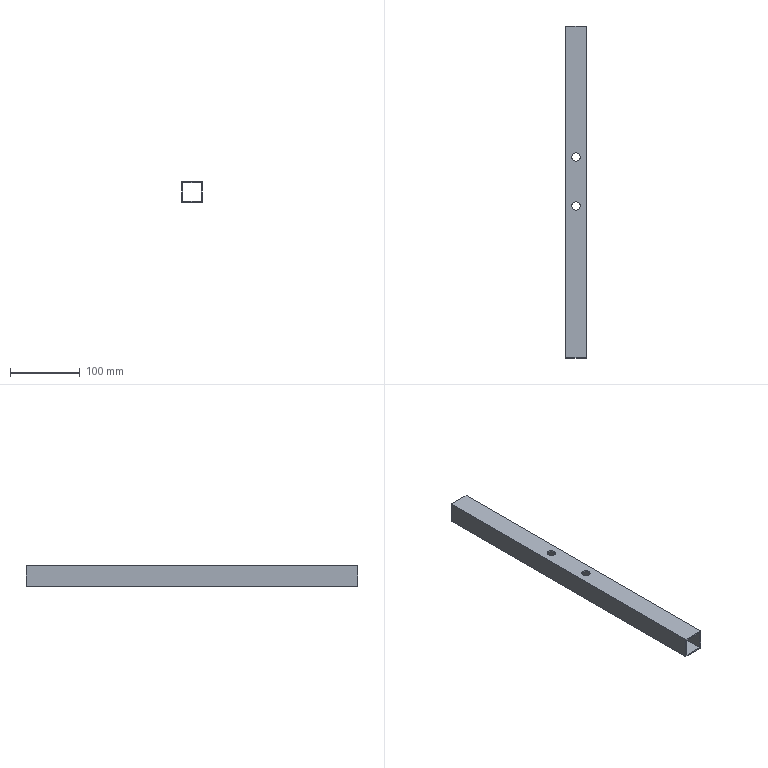Part | NX | features solid 2 | 1 solid | 14 faces | box 30 x 475 x 30 mm | volume 105495 mm3 | plane 10 | cylinder 4 | commonest cylinder face diameters 12 x4
STEP:
#1=CARTESIAN_POINT('',(240.,300.,-15.));
#2=VERTEX_POINT('',#1);
#3=CARTESIAN_POINT('',(270.,300.,-15.));
#4=VERTEX_POINT('',#3);
#5=CARTESIAN_POINT('',(270.,300.,-15.));
#6=DIRECTION('',(-1.,0.,0.));
#7=VECTOR('',#6,1000.);
#8=LINE('',#5,#7);
#9=EDGE_CURVE('',#2,#4,#8,.F.);
#10=ORIENTED_EDGE('',*,*,#9,.F.);
#11=CARTESIAN_POINT('',(240.,-175.,-15.));
#12=VERTEX_POINT('',#11);
#13=CARTESIAN_POINT('',(240.,40.,-15.));
#14=DIRECTION('',(0.,1.,0.));
#15=VECTOR('',#14,1000.);
#16=LINE('',#13,#15);
#17=EDGE_CURVE('',#12,#2,#16,.T.);
#18=ORIENTED_EDGE('',*,*,#17,.F.);
#19=CARTESIAN_POINT('',(270.,-175.,-15.));
#20=VERTEX_POINT('',#19);
#21=CARTESIAN_POINT('',(25.,-175.,-15.));
#22=DIRECTION('',(1.,0.,0.));
#23=VECTOR('',#22,1000.);
#24=LINE('',#21,#23);
#25=EDGE_CURVE('',#20,#12,#24,.F.);
#26=ORIENTED_EDGE('',*,*,#25,.F.);
#27=CARTESIAN_POINT('',(270.,40.,-15.));
#28=DIRECTION('',(0.,1.,0.));
#29=VECTOR('',#28,1000.);
#30=LINE('',#27,#29);
#31=EDGE_CURVE('',#20,#4,#30,.T.);
#32=ORIENTED_EDGE('',*,*,#31,.T.);
#33=EDGE_LOOP('',(#10,#18,#26,#32));
#34=FACE_BOUND('',#33,.T.);
#35=CARTESIAN_POINT('',(249.,112.5,-15.));
#36=VERTEX_POINT('',#35);
#37=CARTESIAN_POINT('',(255.,112.5,-15.));
#38=DIRECTION('',(0.,0.,-1.));
#39=DIRECTION('',(-1.,0.,0.));
#40=AXIS2_PLACEMENT_3D('',#37,#38,#39);
#41=CIRCLE('',#40,6.);
#42=EDGE_CURVE('',#36,#36,#41,.T.);
#43=ORIENTED_EDGE('',*,*,#42,.T.);
#44=EDGE_LOOP('',(#43));
#45=FACE_BOUND('',#44,.T.);
#46=CARTESIAN_POINT('',(249.,42.5,-15.));
#47=VERTEX_POINT('',#46);
#48=CARTESIAN_POINT('',(255.,42.5,-15.));
#49=DIRECTION('',(0.,0.,-1.));
#50=DIRECTION('',(-1.,0.,0.));
#51=AXIS2_PLACEMENT_3D('',#48,#49,#50);
#52=CIRCLE('',#51,6.);
#53=EDGE_CURVE('',#47,#47,#52,.F.);
#54=ORIENTED_EDGE('',*,*,#53,.F.);
#55=EDGE_LOOP('',(#54));
#56=FACE_BOUND('',#55,.T.);
#57=CARTESIAN_POINT('',(270.,40.,-15.));
#58=DIRECTION('',(0.,0.,-1.));
#59=DIRECTION('',(0.,1.,0.));
#60=AXIS2_PLACEMENT_3D('',#57,#58,#59);
#61=PLANE('',#60);
#62=ADVANCED_FACE('',(#34,#45,#56),#61,.F.);
#63=CARTESIAN_POINT('',(240.,-175.,-45.));
#64=VERTEX_POINT('',#63);
#65=CARTESIAN_POINT('',(240.,300.,-45.));
#66=VERTEX_POINT('',#65);
#67=CARTESIAN_POINT('',(240.,40.,-45.));
#68=DIRECTION('',(0.,1.,0.));
#69=VECTOR('',#68,1000.);
#70=LINE('',#67,#69);
#71=EDGE_CURVE('',#64,#66,#70,.T.);
#72=ORIENTED_EDGE('',*,*,#71,.T.);
#73=CARTESIAN_POINT('',(270.,300.,-45.));
#74=VERTEX_POINT('',#73);
#75=CARTESIAN_POINT('',(270.,300.,-45.));
#76=DIRECTION('',(-1.,0.,0.));
#77=VECTOR('',#76,1000.);
#78=LINE('',#75,#77);
#79=EDGE_CURVE('',#74,#66,#78,.T.);
#80=ORIENTED_EDGE('',*,*,#79,.F.);
#81=CARTESIAN_POINT('',(270.,-175.,-45.));
#82=VERTEX_POINT('',#81);
#83=CARTESIAN_POINT('',(270.,40.,-45.));
#84=DIRECTION('',(0.,1.,0.));
#85=VECTOR('',#84,1000.);
#86=LINE('',#83,#85);
#87=EDGE_CURVE('',#82,#74,#86,.T.);
#88=ORIENTED_EDGE('',*,*,#87,.F.);
#89=CARTESIAN_POINT('',(270.,-175.,-45.));
#90=DIRECTION('',(-1.,0.,0.));
#91=VECTOR('',#90,1000.);
#92=LINE('',#89,#91);
#93=EDGE_CURVE('',#82,#64,#92,.T.);
#94=ORIENTED_EDGE('',*,*,#93,.T.);
#95=EDGE_LOOP('',(#72,#80,#88,#94));
#96=FACE_BOUND('',#95,.T.);
#97=CARTESIAN_POINT('',(261.,112.5,-45.));
#98=VERTEX_POINT('',#97);
#99=CARTESIAN_POINT('',(255.,112.5,-45.));
#100=DIRECTION('',(0.,0.,-1.));
#101=DIRECTION('',(1.,0.,0.));
#102=AXIS2_PLACEMENT_3D('',#99,#100,#101);
#103=CIRCLE('',#102,6.);
#104=EDGE_CURVE('',#98,#98,#103,.T.);
#105=ORIENTED_EDGE('',*,*,#104,.F.);
#106=EDGE_LOOP('',(#105));
#107=FACE_BOUND('',#106,.T.);
#108=CARTESIAN_POINT('',(261.,42.5,-45.));
#109=VERTEX_POINT('',#108);
#110=CARTESIAN_POINT('',(255.,42.5,-45.));
#111=DIRECTION('',(0.,0.,1.));
#112=DIRECTION('',(1.,0.,0.));
#113=AXIS2_PLACEMENT_3D('',#110,#111,#112);
#114=CIRCLE('',#113,6.);
#115=EDGE_CURVE('',#109,#109,#114,.T.);
#116=ORIENTED_EDGE('',*,*,#115,.T.);
#117=EDGE_LOOP('',(#116));
#118=FACE_BOUND('',#117,.T.);
#119=CARTESIAN_POINT('',(270.,40.,-45.));
#120=DIRECTION('',(0.,0.,-1.));
#121=DIRECTION('',(0.,1.,0.));
#122=AXIS2_PLACEMENT_3D('',#119,#120,#121);
#123=PLANE('',#122);
#124=ADVANCED_FACE('',(#96,#107,#118),#123,.T.);
#125=CARTESIAN_POINT('',(242.,-175.,-17.));
#126=VERTEX_POINT('',#125);
#127=CARTESIAN_POINT('',(242.,300.,-17.));
#128=VERTEX_POINT('',#127);
#129=CARTESIAN_POINT('',(242.,40.,-17.));
#130=DIRECTION('',(0.,1.,0.));
#131=VECTOR('',#130,1000.);
#132=LINE('',#129,#131);
#133=EDGE_CURVE('',#126,#128,#132,.T.);
#134=ORIENTED_EDGE('',*,*,#133,.T.);
#135=CARTESIAN_POINT('',(268.,300.,-17.));
#136=VERTEX_POINT('',#135);
#137=CARTESIAN_POINT('',(270.,300.,-17.));
#138=DIRECTION('',(-1.,0.,0.));
#139=VECTOR('',#138,1000.);
#140=LINE('',#137,#139);
#141=EDGE_CURVE('',#128,#136,#140,.F.);
#142=ORIENTED_EDGE('',*,*,#141,.T.);
#143=CARTESIAN_POINT('',(268.,-175.,-17.));
#144=VERTEX_POINT('',#143);
#145=CARTESIAN_POINT('',(268.,40.,-17.));
#146=DIRECTION('',(0.,1.,0.));
#147=VECTOR('',#146,1000.);
#148=LINE('',#145,#147);
#149=EDGE_CURVE('',#144,#136,#148,.T.);
#150=ORIENTED_EDGE('',*,*,#149,.F.);
#151=CARTESIAN_POINT('',(25.,-175.,-17.));
#152=DIRECTION('',(1.,0.,0.));
#153=VECTOR('',#152,1000.);
#154=LINE('',#151,#153);
#155=EDGE_CURVE('',#144,#126,#154,.F.);
#156=ORIENTED_EDGE('',*,*,#155,.T.);
#157=EDGE_LOOP('',(#134,#142,#150,#156));
#158=FACE_BOUND('',#157,.T.);
#159=CARTESIAN_POINT('',(249.,112.5,-17.));
#160=VERTEX_POINT('',#159);
#161=CARTESIAN_POINT('',(255.,112.5,-17.));
#162=DIRECTION('',(0.,0.,-1.));
#163=DIRECTION('',(-1.,0.,0.));
#164=AXIS2_PLACEMENT_3D('',#161,#162,#163);
#165=CIRCLE('',#164,6.);
#166=EDGE_CURVE('',#160,#160,#165,.T.);
#167=ORIENTED_EDGE('',*,*,#166,.F.);
#168=EDGE_LOOP('',(#167));
#169=FACE_BOUND('',#168,.T.);
#170=CARTESIAN_POINT('',(249.,42.5,-17.));
#171=VERTEX_POINT('',#170);
#172=CARTESIAN_POINT('',(255.,42.5,-17.));
#173=DIRECTION('',(0.,0.,-1.));
#174=DIRECTION('',(-1.,0.,0.));
#175=AXIS2_PLACEMENT_3D('',#172,#173,#174);
#176=CIRCLE('',#175,6.);
#177=EDGE_CURVE('',#171,#171,#176,.F.);
#178=ORIENTED_EDGE('',*,*,#177,.T.);
#179=EDGE_LOOP('',(#178));
#180=FACE_BOUND('',#179,.T.);
#181=CARTESIAN_POINT('',(270.,40.,-17.));
#182=DIRECTION('',(0.,0.,-1.));
#183=DIRECTION('',(0.,1.,0.));
#184=AXIS2_PLACEMENT_3D('',#181,#182,#183);
#185=PLANE('',#184);
#186=ADVANCED_FACE('',(#158,#169,#180),#185,.T.);
#187=CARTESIAN_POINT('',(268.,-175.,-43.));
#188=VERTEX_POINT('',#187);
#189=CARTESIAN_POINT('',(268.,300.,-43.));
#190=VERTEX_POINT('',#189);
#191=CARTESIAN_POINT('',(268.,40.,-43.));
#192=DIRECTION('',(0.,-1.,0.));
#193=VECTOR('',#192,1000.);
#194=LINE('',#191,#193);
#195=EDGE_CURVE('',#188,#190,#194,.F.);
#196=ORIENTED_EDGE('',*,*,#195,.T.);
#197=CARTESIAN_POINT('',(242.,300.,-43.));
#198=VERTEX_POINT('',#197);
#199=CARTESIAN_POINT('',(270.,300.,-43.));
#200=DIRECTION('',(-1.,0.,0.));
#201=VECTOR('',#200,1000.);
#202=LINE('',#199,#201);
#203=EDGE_CURVE('',#190,#198,#202,.T.);
#204=ORIENTED_EDGE('',*,*,#203,.T.);
#205=CARTESIAN_POINT('',(242.,-175.,-43.));
#206=VERTEX_POINT('',#205);
#207=CARTESIAN_POINT('',(242.,40.,-43.));
#208=DIRECTION('',(0.,-1.,0.));
#209=VECTOR('',#208,1000.);
#210=LINE('',#207,#209);
#211=EDGE_CURVE('',#206,#198,#210,.F.);
#212=ORIENTED_EDGE('',*,*,#211,.F.);
#213=CARTESIAN_POINT('',(270.,-175.,-43.));
#214=DIRECTION('',(-1.,0.,0.));
#215=VECTOR('',#214,1000.);
#216=LINE('',#213,#215);
#217=EDGE_CURVE('',#188,#206,#216,.T.);
#218=ORIENTED_EDGE('',*,*,#217,.F.);
#219=EDGE_LOOP('',(#196,#204,#212,#218));
#220=FACE_BOUND('',#219,.T.);
#221=CARTESIAN_POINT('',(249.,112.5,-43.));
#222=VERTEX_POINT('',#221);
#223=CARTESIAN_POINT('',(255.,112.5,-43.));
#224=DIRECTION('',(0.,0.,-1.));
#225=DIRECTION('',(-1.,0.,0.));
#226=AXIS2_PLACEMENT_3D('',#223,#224,#225);
#227=CIRCLE('',#226,6.);
#228=EDGE_CURVE('',#222,#222,#227,.F.);
#229=ORIENTED_EDGE('',*,*,#228,.F.);
#230=EDGE_LOOP('',(#229));
#231=FACE_BOUND('',#230,.T.);
#232=CARTESIAN_POINT('',(249.,42.5,-43.));
#233=VERTEX_POINT('',#232);
#234=CARTESIAN_POINT('',(255.,42.5,-43.));
#235=DIRECTION('',(0.,0.,-1.));
#236=DIRECTION('',(-1.,0.,0.));
#237=AXIS2_PLACEMENT_3D('',#234,#235,#236);
#238=CIRCLE('',#237,6.);
#239=EDGE_CURVE('',#233,#233,#238,.T.);
#240=ORIENTED_EDGE('',*,*,#239,.T.);
#241=EDGE_LOOP('',(#240));
#242=FACE_BOUND('',#241,.T.);
#243=CARTESIAN_POINT('',(270.,40.,-43.));
#244=DIRECTION('',(0.,0.,-1.));
#245=DIRECTION('',(0.,1.,0.));
#246=AXIS2_PLACEMENT_3D('',#243,#244,#245);
#247=PLANE('',#246);
#248=ADVANCED_FACE('',(#220,#231,#242),#247,.F.);
#249=CARTESIAN_POINT('',(242.,300.,-45.));
#250=DIRECTION('',(0.,0.,-1.));
#251=VECTOR('',#250,1000.);
#252=LINE('',#249,#251);
#253=EDGE_CURVE('',#198,#128,#252,.F.);
#254=ORIENTED_EDGE('',*,*,#253,.F.);
#255=ORIENTED_EDGE('',*,*,#203,.F.);
#256=CARTESIAN_POINT('',(268.,300.,-45.));
#257=DIRECTION('',(0.,0.,-1.));
#258=VECTOR('',#257,1000.);
#259=LINE('',#256,#258);
#260=EDGE_CURVE('',#190,#136,#259,.F.);
#261=ORIENTED_EDGE('',*,*,#260,.T.);
#262=ORIENTED_EDGE('',*,*,#141,.F.);
#263=EDGE_LOOP('',(#254,#255,#261,#262));
#264=FACE_BOUND('',#263,.T.);
#265=ORIENTED_EDGE('',*,*,#79,.T.);
#266=CARTESIAN_POINT('',(240.,300.,-45.));
#267=DIRECTION('',(0.,0.,-1.));
#268=VECTOR('',#267,1000.);
#269=LINE('',#266,#268);
#270=EDGE_CURVE('',#66,#2,#269,.F.);
#271=ORIENTED_EDGE('',*,*,#270,.T.);
#272=ORIENTED_EDGE('',*,*,#9,.T.);
#273=CARTESIAN_POINT('',(270.,300.,-45.));
#274=DIRECTION('',(0.,0.,-1.));
#275=VECTOR('',#274,1000.);
#276=LINE('',#273,#275);
#277=EDGE_CURVE('',#74,#4,#276,.F.);
#278=ORIENTED_EDGE('',*,*,#277,.F.);
#279=EDGE_LOOP('',(#265,#271,#272,#278));
#280=FACE_BOUND('',#279,.T.);
#281=CARTESIAN_POINT('',(35.,300.,-45.));
#282=DIRECTION('',(0.,-1.,0.));
#283=DIRECTION('',(1.,0.,0.));
#284=AXIS2_PLACEMENT_3D('',#281,#282,#283);
#285=PLANE('',#284);
#286=ADVANCED_FACE('',(#264,#280),#285,.F.);
#287=ORIENTED_EDGE('',*,*,#270,.F.);
#288=ORIENTED_EDGE('',*,*,#71,.F.);
#289=CARTESIAN_POINT('',(240.,-175.,-45.));
#290=DIRECTION('',(0.,0.,-1.));
#291=VECTOR('',#290,1000.);
#292=LINE('',#289,#291);
#293=EDGE_CURVE('',#64,#12,#292,.F.);
#294=ORIENTED_EDGE('',*,*,#293,.T.);
#295=ORIENTED_EDGE('',*,*,#17,.T.);
#296=EDGE_LOOP('',(#287,#288,#294,#295));
#297=FACE_BOUND('',#296,.T.);
#298=CARTESIAN_POINT('',(240.,40.,-45.));
#299=DIRECTION('',(1.,0.,0.));
#300=DIRECTION('',(0.,1.,0.));
#301=AXIS2_PLACEMENT_3D('',#298,#299,#300);
#302=PLANE('',#301);
#303=ADVANCED_FACE('',(#297),#302,.F.);
#304=ORIENTED_EDGE('',*,*,#87,.T.);
#305=ORIENTED_EDGE('',*,*,#277,.T.);
#306=ORIENTED_EDGE('',*,*,#31,.F.);
#307=CARTESIAN_POINT('',(270.,-175.,-45.));
#308=DIRECTION('',(0.,0.,-1.));
#309=VECTOR('',#308,1000.);
#310=LINE('',#307,#309);
#311=EDGE_CURVE('',#82,#20,#310,.F.);
#312=ORIENTED_EDGE('',*,*,#311,.F.);
#313=EDGE_LOOP('',(#304,#305,#306,#312));
#314=FACE_BOUND('',#313,.T.);
#315=CARTESIAN_POINT('',(270.,40.,-45.));
#316=DIRECTION('',(1.,0.,0.));
#317=DIRECTION('',(0.,1.,0.));
#318=AXIS2_PLACEMENT_3D('',#315,#316,#317);
#319=PLANE('',#318);
#320=ADVANCED_FACE('',(#314),#319,.T.);
#321=ORIENTED_EDGE('',*,*,#311,.T.);
#322=ORIENTED_EDGE('',*,*,#25,.T.);
#323=ORIENTED_EDGE('',*,*,#293,.F.);
#324=ORIENTED_EDGE('',*,*,#93,.F.);
#325=EDGE_LOOP('',(#321,#322,#323,#324));
#326=FACE_BOUND('',#325,.T.);
#327=CARTESIAN_POINT('',(268.,-175.,-45.));
#328=DIRECTION('',(0.,0.,-1.));
#329=VECTOR('',#328,1000.);
#330=LINE('',#327,#329);
#331=EDGE_CURVE('',#188,#144,#330,.F.);
#332=ORIENTED_EDGE('',*,*,#331,.F.);
#333=ORIENTED_EDGE('',*,*,#217,.T.);
#334=CARTESIAN_POINT('',(242.,-175.,-45.));
#335=DIRECTION('',(0.,0.,-1.));
#336=VECTOR('',#335,1000.);
#337=LINE('',#334,#336);
#338=EDGE_CURVE('',#206,#126,#337,.F.);
#339=ORIENTED_EDGE('',*,*,#338,.T.);
#340=ORIENTED_EDGE('',*,*,#155,.F.);
#341=EDGE_LOOP('',(#332,#333,#339,#340));
#342=FACE_BOUND('',#341,.T.);
#343=CARTESIAN_POINT('',(25.,-175.,-75.));
#344=DIRECTION('',(0.,-1.,0.));
#345=DIRECTION('',(1.,0.,0.));
#346=AXIS2_PLACEMENT_3D('',#343,#344,#345);
#347=PLANE('',#346);
#348=ADVANCED_FACE('',(#326,#342),#347,.T.);
#349=ORIENTED_EDGE('',*,*,#260,.F.);
#350=ORIENTED_EDGE('',*,*,#195,.F.);
#351=ORIENTED_EDGE('',*,*,#331,.T.);
#352=ORIENTED_EDGE('',*,*,#149,.T.);
#353=EDGE_LOOP('',(#349,#350,#351,#352));
#354=FACE_BOUND('',#353,.T.);
#355=CARTESIAN_POINT('',(268.,40.,-45.));
#356=DIRECTION('',(1.,0.,0.));
#357=DIRECTION('',(0.,1.,0.));
#358=AXIS2_PLACEMENT_3D('',#355,#356,#357);
#359=PLANE('',#358);
#360=ADVANCED_FACE('',(#354),#359,.F.);
#361=ORIENTED_EDGE('',*,*,#211,.T.);
#362=ORIENTED_EDGE('',*,*,#253,.T.);
#363=ORIENTED_EDGE('',*,*,#133,.F.);
#364=ORIENTED_EDGE('',*,*,#338,.F.);
#365=EDGE_LOOP('',(#361,#362,#363,#364));
#366=FACE_BOUND('',#365,.T.);
#367=CARTESIAN_POINT('',(242.,40.,-45.));
#368=DIRECTION('',(1.,0.,0.));
#369=DIRECTION('',(0.,1.,0.));
#370=AXIS2_PLACEMENT_3D('',#367,#368,#369);
#371=PLANE('',#370);
#372=ADVANCED_FACE('',(#366),#371,.T.);
#373=ORIENTED_EDGE('',*,*,#228,.T.);
#374=EDGE_LOOP('',(#373));
#375=FACE_BOUND('',#374,.T.);
#376=ORIENTED_EDGE('',*,*,#104,.T.);
#377=EDGE_LOOP('',(#376));
#378=FACE_BOUND('',#377,.T.);
#379=CARTESIAN_POINT('',(255.,112.5,255.));
#380=DIRECTION('',(0.,0.,-1.));
#381=DIRECTION('',(-1.,0.,0.));
#382=AXIS2_PLACEMENT_3D('',#379,#380,#381);
#383=CYLINDRICAL_SURFACE('',#382,6.);
#384=ADVANCED_FACE('',(#375,#378),#383,.F.);
#385=ORIENTED_EDGE('',*,*,#166,.T.);
#386=EDGE_LOOP('',(#385));
#387=FACE_BOUND('',#386,.T.);
#388=ORIENTED_EDGE('',*,*,#42,.F.);
#389=EDGE_LOOP('',(#388));
#390=FACE_BOUND('',#389,.T.);
#391=CARTESIAN_POINT('',(255.,112.5,255.));
#392=DIRECTION('',(0.,0.,-1.));
#393=DIRECTION('',(-1.,0.,0.));
#394=AXIS2_PLACEMENT_3D('',#391,#392,#393);
#395=CYLINDRICAL_SURFACE('',#394,6.);
#396=ADVANCED_FACE('',(#387,#390),#395,.F.);
#397=ORIENTED_EDGE('',*,*,#239,.F.);
#398=EDGE_LOOP('',(#397));
#399=FACE_BOUND('',#398,.T.);
#400=ORIENTED_EDGE('',*,*,#115,.F.);
#401=EDGE_LOOP('',(#400));
#402=FACE_BOUND('',#401,.T.);
#403=CARTESIAN_POINT('',(255.,42.5,255.));
#404=DIRECTION('',(0.,0.,-1.));
#405=DIRECTION('',(-1.,0.,0.));
#406=AXIS2_PLACEMENT_3D('',#403,#404,#405);
#407=CYLINDRICAL_SURFACE('',#406,6.);
#408=ADVANCED_FACE('',(#399,#402),#407,.F.);
#409=ORIENTED_EDGE('',*,*,#177,.F.);
#410=EDGE_LOOP('',(#409));
#411=FACE_BOUND('',#410,.T.);
#412=ORIENTED_EDGE('',*,*,#53,.T.);
#413=EDGE_LOOP('',(#412));
#414=FACE_BOUND('',#413,.T.);
#415=CARTESIAN_POINT('',(255.,42.5,255.));
#416=DIRECTION('',(0.,0.,-1.));
#417=DIRECTION('',(-1.,0.,0.));
#418=AXIS2_PLACEMENT_3D('',#415,#416,#417);
#419=CYLINDRICAL_SURFACE('',#418,6.);
#420=ADVANCED_FACE('',(#411,#414),#419,.F.);
#421=CLOSED_SHELL('',(#62,#124,#186,#248,#286,#303,#320,#348,#360,#372,#384,#396,#408,#420));
#422=MANIFOLD_SOLID_BREP('',#421);
#423=(LENGTH_UNIT()NAMED_UNIT(*)SI_UNIT(.MILLI.,.METRE.));
#424=UNCERTAINTY_MEASURE_WITH_UNIT(LENGTH_MEASURE(0.00001),#423,'','');
#425=(NAMED_UNIT(*)PLANE_ANGLE_UNIT()SI_UNIT($,.RADIAN.));
#426=(NAMED_UNIT(*)SI_UNIT($,.STERADIAN.)SOLID_ANGLE_UNIT());
#427=(GEOMETRIC_REPRESENTATION_CONTEXT(3)GLOBAL_UNCERTAINTY_ASSIGNED_CONTEXT((#424))GLOBAL_UNIT_ASSIGNED_CONTEXT((#423,#425,#426))REPRESENTATION_CONTEXT('',''));
#428=ADVANCED_BREP_SHAPE_REPRESENTATION('',(#422),#427);